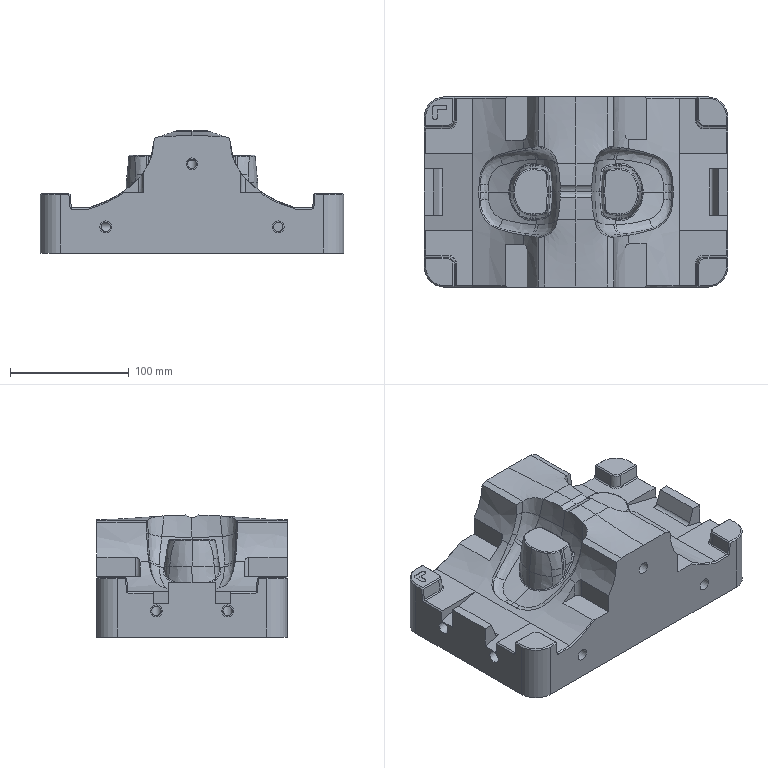NC program | NX | posted with a generic post | part box 255 x 160 x 102.619 mm
Lines 1 to 981 of 55104:
N10 G17 G21 G94 G90
(CAVITY_MILL , TOOL : D30R5)
N12 T00 M6
N14 G54
N16 G17 G0 G90 X177.095 Y-14.998 S1500 M3
N18 G43 Z115. H0
N20 Z102.321
N22 G94 G1 Z102.121 F1800.
N24 Y1.322
N26 X10.431
N28 G2 X1.322 Y10.429 R17.
N30 G1 Y149.575
N32 G2 X10.431 Y158.681 R17.
N34 G1 X244.569
N36 G2 X253.678 Y149.575 R17.
N38 G1 Y10.429
N40 G2 X244.569 Y1.322 R17.
N42 G1 X177.095
N44 Y15.322
N46 X15.322
N48 Y144.681
N50 X239.678
N52 Y15.322
N54 X177.095
N56 Y29.322
N58 X29.322
N60 Y130.681
N62 X225.678
N64 Y29.322
N66 X177.095
N68 Y43.322
N70 X43.322
N72 Y116.681
N74 X98.445
N76 Y102.681
N78 G3 X98.293 Y97.004 R56.063
N80 G1 X98.589 Y84.666
N82 G3 X99.438 Y79.957 R15.536
N84 X98.536 Y73.276 R18.646
N86 X98.46 Y57.322 R148.96
N88 G1 X57.322
N90 Y102.681
N92 X98.445
N94 X84.488 Y88.681
N96 X84.593 Y84.33
N98 G3 X85.029 Y79.931 R29.536
N100 X84.523 Y73.439 R32.646
N102 X84.422 Y71.322 R162.96
N104 G1 X71.322
N106 Y88.681
N108 X84.488
N110 X98.445 Y102.681
N112 Y116.681
N114 X211.678
N116 Y43.322
N118 X177.095
N120 Y57.322
N122 X156.555
N124 G3 X156.707 Y62.999 R56.064
N126 G1 X156.411 Y75.338
N128 G3 X155.562 Y80.046 R15.536
N130 X156.464 Y86.727 R18.646
N132 X156.538 Y102.681 R148.12
N134 G1 X153.741 Y102.543
N136 G2 X153.659 Y86.737 R145.32
N138 X152.574 Y80.012 R15.846
N140 X153.612 Y75.271 R12.736
N142 G1 X153.908 Y62.932
N144 G2 X153.69 Y56.679 R53.264
N146 X142.632 Y46.609 R11.109
N148 G1 X112.375 Y46.603
N150 G2 X101.272 Y57.153 R11.115
N152 X101.341 Y73.266 R146.16
N154 X102.426 Y79.991 R15.846
N156 X101.388 Y84.733 R12.736
N158 G1 X101.092 Y97.071
N160 G2 X101.31 Y103.324 R53.263
N162 X112.369 Y113.394 R11.108
N164 G1 X142.63 Y113.398
N166 G2 X153.726 Y102.859 R11.109
N168 X153.741 Y102.543 R145.32
N170 G1 X156.538 Y102.681
N172 X197.678
N174 Y57.322
N176 X177.095
N178 Y71.322
N180 X170.512
N182 X170.407 Y75.673
N184 G3 X169.971 Y80.072 R29.536
N186 X170.477 Y86.563 R32.646
N188 X170.578 Y88.681 R162.12
N190 G1 X183.678
N192 Y71.322
N194 X177.095
N196 Y56.322
N198 Z102.321
N200 G0 Z102.92
N202 Y-14.998
N204 Z101.821
N206 G1 Z101.621
N208 Y0.502
N210 X12.905
N212 G2 X0.502 Y12.901 R17.
N214 G1 Y147.103
N216 G2 X12.905 Y159.501 R17.
N218 G1 X242.095
N220 G2 X254.498 Y147.103 R17.
N222 G1 Y12.901
N224 G2 X242.095 Y0.502 R17.
N226 G1 X177.095
N228 Y14.502
N230 X15.341
N232 G2 X14.502 Y15.34 R3.
N234 G1 Y144.663
N236 G2 X15.341 Y145.501 R3.
N238 G1 X239.659
N240 G2 X240.498 Y144.663 R3.
N242 G1 Y15.34
N244 G2 X239.659 Y14.502 R3.
N246 G1 X177.095
N248 Y28.502
N250 X28.502
N252 Y131.501
N254 X101.002
N256 Y117.501
N258 G3 X96.735 Y106.436 R15.365
N260 G1 X96.799 Y104.162
N262 X96.803 Y104.064
N264 G2 X97.893 Y84.247 R872.408
N266 G3 X98.673 Y79.993 R15.74
N268 X97.894 Y75.752 R15.657
N270 G1 X97.557 Y68.018
N272 X97.482 Y66.698
N274 X96.8 Y55.879
N276 X96.797 Y55.778
N278 X96.772 Y52.822
N280 G3 X100.983 Y42.502 R14.442
N282 G1 X42.502
N284 Y117.501
N286 X101.002
N288 X82.814 Y103.501
N290 X82.825 Y103.27
N292 G2 X83.906 Y83.638 R858.408
N294 G3 X84.29 Y79.995 R29.74
N296 X83.907 Y76.36 R29.657
N298 G1 X83.507 Y67.537
N300 X82.831 Y56.811
N302 G3 X82.814 Y56.502 R16.8
N304 G1 X73.422
N306 Y66.502
N308 X66.502
N310 Y93.501
N312 X73.404
N314 G2 X73.915 Y83.202 R848.408
N316 G3 X74.186 Y79.995 R39.74
N318 X73.917 Y76.805 R39.657
N320 G1 X73.521 Y68.078
N322 X73.422 Y66.502
N324 Y56.502
N326 X56.502
N328 Y103.501
N330 X82.814
N332 X101.002 Y117.501
N334 Y131.501
N336 X226.498
N338 Y28.502
N340 X177.095
N342 Y42.502
N344 X153.998
N346 G3 X158.265 Y53.567 R15.365
N348 G1 X158.201 Y55.841
N350 X158.197 Y55.939
N352 G2 X157.107 Y75.756 R872.408
N354 G3 X156.327 Y80.01 R15.74
N356 X157.106 Y84.251 R15.657
N358 G1 X157.443 Y91.984
N360 X157.519 Y93.304
N362 X158.2 Y104.124
N364 X158.203 Y104.225
N366 X158.228 Y107.18
N368 G3 X154.017 Y117.501 R14.443
N370 G1 X152.033 Y115.525
N372 G2 X155.428 Y107.205 R11.643
N374 G1 X155.403 Y104.249
N376 X154.724 Y93.472
N378 X154.647 Y92.125
N380 X154.309 Y84.373
N382 G2 X153.342 Y80.011 R12.857
N384 X154.31 Y75.634 R12.94
N386 G3 X155.403 Y55.754 R875.208
N388 G1 X155.466 Y53.489
N390 G2 X150.436 Y43.076 R12.565
N392 X141.06 Y40.312 R24.234
N394 G1 X134.577 Y39.769
N396 G2 X108.878 Y41.291 R90.461
N398 X99.572 Y52.798 R11.642
N400 G1 X99.597 Y55.754
N402 X100.277 Y66.531
N404 X100.353 Y67.878
N406 X100.691 Y75.63
N408 G2 X101.658 Y79.992 R12.857
N410 X100.69 Y84.369 R12.94
N412 G3 X99.597 Y104.249 R875.208
N414 G1 X99.534 Y106.515
N416 G2 X104.564 Y116.927 R12.565
N418 X114.012 Y119.695 R24.228
N420 G1 X120.96 Y120.254
N422 G2 X146.132 Y118.71 R89.338
N424 X152.033 Y115.525 R11.643
N426 G1 X154.017 Y117.501
N428 X212.498
N430 Y42.502
N432 X177.095
N434 Y56.502
N436 X172.186
N438 X172.175 Y56.733
N440 G2 X171.094 Y76.365 R858.408
N442 G3 X170.71 Y80.008 R29.74
N444 X171.093 Y83.642 R29.657
N446 G1 X171.494 Y92.462
N448 X172.169 Y103.193
N450 G3 X172.186 Y103.501 R16.8
N452 G1 X198.498
N454 Y93.501
N456 X188.498
N458 Y66.502
N460 X181.596
N462 G2 X181.085 Y76.801 R848.408
N464 G3 X180.814 Y80.008 R39.74
N466 X181.083 Y83.197 R39.657
N468 G1 X181.48 Y91.921
N470 X181.579 Y93.501
N472 X188.498
N474 X198.498
N476 Y56.502
N478 X177.095
N480 Y41.502
N482 Z101.821
N484 G0 Z102.421
N486 Y-14.998
N488 Z101.322
N490 G1 Z101.122
N492 Y0.002
N494 X17.
N496 G2 X0. Y17.002 R17.
N498 G1 Y143.002
N500 G2 X17. Y160.002 R17.
N502 G1 X238.
N504 G2 X255. Y143.002 R17.
N506 G1 Y17.002
N508 G2 X238. Y0.002 R17.
N510 G1 X177.095
N512 Y14.002
N514 X17.
N516 G2 X14. Y17.002 R3.
N518 G1 Y143.002
N520 G2 X17. Y146.002 R3.
N522 G1 X238.
N524 G2 X241. Y143.002 R3.
N526 G1 Y17.002
N528 G2 X238. Y14.002 R3.
N530 G1 X177.095
N532 Y28.002
N534 X28.
N536 Y132.002
N538 X97.508
N540 Y118.002
N542 G3 X95.334 Y107.532 R15.873
N544 G2 X97.346 Y84.42 R222.849
N546 G3 X98.109 Y79.993 R16.551
N548 X97.346 Y75.576 R16.485
N550 G2 X95.335 Y52.474 R222.602
N552 G3 X97.508 Y42.002 R15.875
N554 G1 X42.
N556 Y118.002
N558 X97.508
N560 X81.685 Y104.002
N562 G2 X83.354 Y83.934 R208.849
N564 G3 X83.748 Y79.995 R30.551
N566 X83.355 Y76.062 R30.485
N568 G2 X82.687 Y65.13 R208.602
N570 G1 X72.725 Y66.002
N572 X66.
N574 Y94.002
N576 X72.724
N578 G2 X73.36 Y83.587 R198.849
N580 G3 X73.645 Y79.995 R40.551
N582 X73.361 Y76.41 R40.485
N584 G2 X72.725 Y66.002 R198.602
N586 G1 X82.687 Y65.13
N588 G2 X81.686 Y56.002 R208.602
N590 G1 X56.
N592 Y104.002
N594 X81.685
N596 X97.508 Y118.002
N598 Y132.002
N600 X227.
N602 Y28.002
N604 X177.095
N606 Y42.002
N608 X157.492
N610 G3 X159.666 Y52.471 R15.873
N612 G2 X157.654 Y75.583 R222.848
N614 G3 X156.891 Y80.01 R16.552
N616 X157.654 Y84.427 R16.49
N618 G2 X159.665 Y107.53 R222.815
N620 G3 X157.492 Y118.002 R15.875
N622 G1 X155.102 Y116.542
N624 G2 X156.892 Y107.918 R13.075
N626 G3 X154.856 Y84.524 R225.615
N628 G2 X153.922 Y80.011 R13.69
N630 X154.856 Y75.486 R13.752
N632 G3 X156.893 Y52.084 R225.648
N634 G2 X153.094 Y40.936 R13.073
N636 X124.802 Y33.091 R49.203
N638 X101.906 Y40.936 R50.384
N640 X98.108 Y52.086 R13.075
N642 G3 X100.145 Y75.479 R225.402
N644 G2 X101.078 Y79.992 R13.685
N646 X100.144 Y84.518 R13.751
N648 G3 X98.107 Y107.919 R225.649
N650 G2 X101.906 Y119.067 R13.073
N652 X130.198 Y126.913 R49.203
N654 X153.094 Y119.067 R50.354
N656 X155.102 Y116.542 R13.075
N658 G1 X157.492 Y118.002
N660 X213.
N662 Y42.002
N664 X177.095
N666 Y56.002
N668 X173.315
N670 G2 X171.646 Y76.069 R208.848
N672 G3 X171.252 Y80.009 R30.552
N674 X171.645 Y83.94 R30.49
N676 G2 X173.314 Y104.002 R208.815
N678 G1 X199.
N680 Y56.002
N682 X189.
N684 Y66.002
N686 X182.276
N688 G2 X181.64 Y76.416 R198.848
N690 G3 X181.355 Y80.009 R40.552
N692 X181.639 Y83.592 R40.49
N694 G2 X182.275 Y94.002 R198.815
N696 G1 X189.
N698 Y66.002
N700 Y56.002
N702 X177.095
N704 Y41.002
N706 Z101.322
N708 G0 Z101.921
N710 Y-14.998
N712 Z100.823
N714 G1 Z100.623
N716 Y0.002
N718 X17.
N720 G2 X0. Y17.002 R17.
N722 G1 Y143.002
N724 G2 X17. Y160.002 R17.
N726 G1 X238.
N728 G2 X255. Y143.002 R17.
N730 G1 Y17.002
N732 G2 X238. Y0.002 R17.
N734 G1 X177.095
N736 Y14.002
N738 X17.
N740 G2 X14. Y17.002 R3.
N742 G1 Y143.002
N744 G2 X17. Y146.002 R3.
N746 G1 X112.205
N748 Y132.002
N750 G3 X99.377 Y123.983 R57.105
N752 X94.053 Y108.951 R15.535
N754 G1 X95.365 Y102.435
N756 G2 X96.953 Y84.27 R187.108
N758 G3 X97.688 Y79.993 R16.509
N760 X96.953 Y75.712 R16.413
N762 G2 X95.521 Y58.803 R179.834
N764 G1 X95.362 Y57.559
N766 X94.275 Y52.233
N768 X94.023 Y50.9
N770 G3 X97.579 Y37.734 R15.35
N772 X97.787 Y37.522 R2.8
N774 X112.166 Y28.002 R55.65
N776 G1 X122.48 Y24.221
N778 X112.166 Y28.002
N780 X28.
N782 Y132.002
N784 X112.205
N786 X122.531 Y135.778
N788 X112.205 Y132.002
N790 X80.361 Y118.002
N792 G3 X80.329 Y106.189 R29.535
N794 G1 X81.552 Y100.112
N796 G2 X82.963 Y83.732 R173.108
N798 G3 X83.338 Y79.994 R30.509
N800 X82.963 Y76.234 R30.413
N802 G2 X81.638 Y60.61 R165.834
N804 G1 X81.541 Y59.85
N806 X80.556 Y55.022
N808 X80.528 Y54.882
N810 X80.277 Y53.555
N812 G3 X80.327 Y42.002 R29.35
N814 G1 X42.
N816 Y118.002
N818 X80.361
N820 X66.492 Y104.002
N822 G3 X66.604 Y103.427 R43.535
N824 G1 X67.735 Y97.806
N826 G2 X68.973 Y83.194 R159.108
N828 G3 X69.212 Y79.994 R44.509
N830 X68.972 Y76.756 R44.413
N832 G2 X67.755 Y62.419 R151.834
N834 G1 X67.72 Y62.141
N836 X66.828 Y57.772
N838 X66.781 Y57.532
N840 X66.529 Y56.199
N842 X66.491 Y56.002
N844 X56.
N846 Y104.002
N848 X66.492
N850 X80.361 Y118.002
N852 X112.205 Y132.002
N854 Y146.002
N856 X238.
N858 G2 X241. Y143.002 R3.
N860 G1 Y17.002
N862 G2 X238. Y14.002 R3.
N864 G1 X177.095
N866 Y28.002
N868 X142.811
N870 X132.494 Y24.223
N872 X142.811 Y28.002
N874 G3 X155.952 Y36.341 R56.515
N876 X161.141 Y49.622 R15.015
N878 G1 X161.008 Y50.707
N880 G3 X160.973 Y50.918 R2.8
N882 G1 X159.635 Y57.568
N884 G2 X158.047 Y75.733 R187.108
N886 G3 X157.312 Y80.011 R16.51
N888 X158.047 Y84.297 R16.483
N890 G2 X159.479 Y101.2 R181.155
N892 G1 X159.638 Y102.444
N894 X160.725 Y107.771
N896 X160.977 Y109.104
N898 G3 X157.421 Y122.269 R15.35
N900 X157.212 Y122.482 R2.8
N902 X142.827 Y132.002 R55.664
N904 G1 X132.509 Y135.782
N906 X142.827 Y132.002
N908 X141.662 Y129.455
N910 G2 X155.324 Y120.414 R52.864
N912 X158.228 Y109.638 R12.55
N914 G1 X157.974 Y108.29
N916 X156.874 Y102.902
N918 X156.702 Y101.555
N920 G3 X155.249 Y84.403 R183.955
N922 G2 X154.349 Y80.012 R13.683
N924 X155.249 Y75.626 R13.71
N926 G3 X156.873 Y57.101 R189.908
N928 G1 X158.229 Y50.366
N930 X158.362 Y49.281
N932 G2 X154.141 Y38.476 R12.215
N934 X127.5 Y26.335 R53.715
N936 X99.676 Y39.589 R52.85
N938 X96.772 Y50.366 R12.55
N940 G1 X97.026 Y51.713
N942 X98.126 Y57.101
N944 X98.298 Y58.448
N946 G3 X99.751 Y75.607 R182.634
N948 G2 X100.651 Y79.991 R13.613
N950 X99.751 Y84.377 R13.709
N952 G3 X98.127 Y102.902 R189.908
N954 G1 X96.798 Y109.504
N956 G2 X101.162 Y121.827 R12.735
N958 X127.5 Y133.663 R54.305
N960 X141.662 Y129.455 R52.864
N962 G1 X142.827 Y132.002
N964 X227.
N966 Y28.002
N968 X177.095
N970 Y42.002
N972 X174.67
N974 G3 X175.036 Y51.331 R29.015
N976 G1 X174.903 Y52.415
N978 G3 X174.698 Y53.68 R16.8
N980 G1 X173.448 Y59.891
N982 G2 X172.037 Y76.271 R173.108
N984 G3 X171.662 Y80.011 R30.51
N986 X172.037 Y83.77 R30.483
N988 G2 X173.362 Y99.396 R167.155
N990 G1 X173.459 Y100.153
N992 X174.444 Y104.98
N994 X174.472 Y105.121
N996 X174.723 Y106.448
N998 G3 X174.673 Y118.002 R29.35
N1000 G1 X213.
N1002 Y42.002
N1004 X177.095
N1006 X188.508 Y56.002
N1008 G3 X188.423 Y56.442 R30.8
N1010 G1 X187.265 Y62.197
N1012 G2 X186.027 Y76.809 R159.108
N1014 G3 X185.788 Y80.012 R44.51
N1016 X186.027 Y83.243 R44.483
N1018 G2 X187.245 Y97.59 R153.155
N1020 G1 X187.28 Y97.863
N1022 X188.172 Y102.23
N1024 X188.219 Y102.471
N1026 X188.471 Y103.804
N1028 X188.509 Y104.002
N1030 X199.
N1032 Y56.002
N1034 X188.508
N1036 Y41.002
N1038 Z100.823
N1040 G0 Z101.422
N1042 X177.095 Y-14.998
N1044 Z100.324
N1046 G1 Z100.124
N1048 Y0.002
N1050 X17.
N1052 G2 X0. Y17.002 R17.
N1054 G1 Y143.002
N1056 G2 X17. Y160.002 R17.
N1058 G1 X238.
N1060 G2 X255. Y143.002 R17.
N1062 G1 Y17.002
N1064 G2 X238. Y0.002 R17.
N1066 G1 X177.095
N1068 Y14.002
N1070 X17.
N1072 G2 X14. Y17.002 R3.
N1074 G1 Y143.002
N1076 G2 X17. Y146.002 R3.
N1078 G1 X103.851
N1080 Y132.002
N1082 G3 X93.864 Y120.584 R52.059
N1084 X93.638 Y120.158 R2.8
N1086 X93.408 Y107.403 R17.11
N1088 G2 X95.051 Y101.167 R30.354
N1090 X96.641 Y84.283 R148.196
N1092 G3 X97.368 Y79.978 R16.747
N1094 X96.626 Y75.493 R18.
N1096 G2 X94.859 Y57.615 R147.007
N1098 X93.447 Y52.701 R36.526
N1100 G3 X93.638 Y39.845 R17.11
N1102 X93.864 Y39.419 R2.8
N1104 X103.851 Y28.002 R52.111
N1106 G1 X28.
N1108 Y132.002
N1110 X103.851
N1112 X78.615 Y118.002
N1114 G3 X80.325 Y102.419 R31.11
N1116 G2 X81.21 Y99.059 R16.354
N1118 X82.65 Y83.77 R134.196
N1120 G3 X83.029 Y79.958 R30.747
N1122 X82.636 Y76.016 R32.
N1124 G2 X81.098 Y60.221 R133.007
N1126 X80.331 Y57.6 R22.526
N1128 G3 X78.615 Y42.002 R31.11
N1130 G1 X42.
N1132 Y118.002
N1134 X78.615
N1136 X65.297 Y104.002
N1138 G3 X67.242 Y97.435 R45.11
N1140 G2 X67.37 Y96.951 R2.354
N1142 X68.659 Y83.257 R120.196
N1144 G3 X68.902 Y79.964 R44.747
N1146 X68.646 Y76.539 R46.
N1148 G2 X67.357 Y62.97 R119.007
N1150 X67.188 Y62.424 R8.526
N1152 G3 X65.297 Y56.002 R45.11
N1154 G1 X56.
N1156 Y104.002
N1158 X65.297
N1160 X78.615 Y118.002
N1162 X103.851 Y132.002
N1164 Y146.002
N1166 X238.
N1168 G2 X241. Y143.002 R3.
N1170 G1 Y17.002
N1172 G2 X238. Y14.002 R3.
N1174 G1 X177.095
N1176 Y28.002
N1178 X151.151
N1180 G3 X161.136 Y39.419 R52.093
N1182 X161.362 Y39.845 R2.8
N1184 X161.592 Y52.6 R17.11
N1186 G2 X159.949 Y58.837 R30.36
N1188 X158.359 Y75.72 R148.196
N1190 G3 X157.636 Y80.012 R16.747
N1192 X158.36 Y84.301 R16.829
N1194 G2 X160.141 Y102.39 R150.257
N1196 X161.553 Y107.302 R36.547
N1198 G3 X161.362 Y120.158 R17.11
N1200 X161.136 Y120.584 R2.8
N1202 X151.147 Y132.002 R52.078
N1204 G1 X149.331 Y129.871
N1206 G2 X158.783 Y119.067 R49.278
N1208 X158.933 Y108.29 R14.31
N1210 G3 X157.387 Y102.902 R39.347
N1212 X155.562 Y84.406 R153.057
N1214 G2 X154.68 Y80.011 R14.029
N1216 X155.561 Y75.617 R13.947
N1218 G3 X157.181 Y58.415 R150.996
N1220 X158.975 Y51.604 R33.16
N1222 G2 X158.783 Y40.936 R14.31
N1224 X127.5 Y19.402 R49.293
N1226 X96.217 Y40.936 R49.311
N1228 X96.067 Y51.713 R14.31
N1230 G3 X97.613 Y57.101 R39.326
N1232 X99.424 Y75.389 R149.807
N1234 G2 X100.32 Y79.992 R15.2
N1236 X99.439 Y84.386 R13.947
N1238 G3 X97.819 Y101.589 R150.996
N1240 X96.025 Y108.399 R33.154
N1242 G2 X96.217 Y119.067 R14.31
N1244 X127.5 Y140.591 R49.259
N1246 X149.331 Y129.871 R49.278
N1248 G1 X151.147 Y132.002
N1250 X227.
N1252 Y28.002
N1254 X177.095
N1256 Y42.002
N1258 X176.385
N1260 G3 X174.675 Y57.584 R31.11
N1262 G2 X173.79 Y60.945 R16.36
N1264 X172.35 Y76.233 R134.196
N1266 G3 X171.977 Y80.014 R30.747
N1268 X172.35 Y83.774 R30.829
N1270 G2 X173.903 Y99.789 R136.257
N1272 X174.669 Y102.404 R22.547
N1274 G3 X176.385 Y118.002 R31.11
N1276 G1 X213.
N1278 Y42.002
N1280 X177.095
N1282 X189.703 Y56.002
N1284 G3 X187.758 Y62.568 R45.11
N1286 G2 X187.63 Y63.053 R2.36
N1288 X186.341 Y76.746 R120.196
N1290 G3 X186.101 Y80.013 R44.747
N1292 X186.34 Y83.247 R44.829
N1294 G2 X187.645 Y97.041 R122.257
N1296 X187.812 Y97.579 R8.547
N1298 G3 X189.703 Y104.002 R45.11
N1300 G1 X199.
N1302 Y56.002
N1304 X189.703
N1306 Y41.002
N1308 Z100.324
N1310 G0 Z100.923
N1312 X177.095 Y-14.998
N1314 Z99.824
N1316 G1 Z99.624
N1318 Y0.002
N1320 X17.
N1322 G2 X0. Y17.002 R17.
N1324 G1 Y143.002
N1326 G2 X17. Y160.002 R17.
N1328 G1 X113.705
N1330 Y146.002
N1332 G3 X94.061 Y124.96 R50.569
N1334 X90.853 Y113.485 R17.766
N1336 X90.881 Y113.24 R2.8
N1338 X93.279 Y105.771 R25.668
N1340 G2 X94.706 Y101.131 R16.658
N1342 X96.369 Y84.707 R133.423
N1344 G3 X97.124 Y79.992 R18.335
N1346 X96.369 Y75.327 R18.601
N1348 G2 X94.712 Y58.902 R132.904
N1350 X93.29 Y54.267 R16.422
N1352 G3 X91.547 Y49.889 R37.565
N1354 X93.046 Y36.907 R15.603
N1356 X114.003 Y14.002 R52.503
N1358 G1 X17.
N1360 G2 X14. Y17.002 R3.
N1362 G1 Y143.002
N1364 G2 X17. Y146.002 R3.
N1366 G1 X113.705
N1368 X81.925 Y132.002
N1370 G3 X76.887 Y112.515 R31.766
N1372 X77.054 Y111.047 R16.8
N1374 X80.668 Y99.689 R39.668
N1376 G2 X80.879 Y98.935 R2.658
N1378 X82.377 Y84.225 R119.423
N1380 G3 X82.789 Y79.987 R32.335
N1382 X82.378 Y75.833 R32.601
N1384 G2 X80.882 Y61.078 R118.904
N1386 X80.647 Y60.278 R2.422
N1388 G3 X78.243 Y54.249 R51.565
N1390 X80.673 Y30.33 R29.603
N1392 X81.857 Y28.002 R66.503
N1394 G1 X28.
N1396 Y132.002
N1398 X81.925
N1400 X62.928 Y118.002
N1402 G3 X62.92 Y111.544 R45.766
N1404 X63.227 Y108.854 R30.8
N1406 X67.29 Y95.241 R53.668
N1408 G2 X68.386 Y83.725 R105.423
N1410 G3 X68.659 Y79.987 R46.335
N1412 X68.388 Y76.348 R46.601
N1414 G2 X67.285 Y64.722 R104.904
N1416 G3 X64.939 Y58.608 R65.565
N1418 X63.14 Y50.7 R43.603
N1420 G1 X53.225 Y52.002
N1422 X52.
N1424 Y108.002
N1426 X53.243
N1428 G3 X53.35 Y107.287 R40.8
N1430 X57.584 Y92.481 R63.668
N1432 G2 X58.393 Y83.36 R95.423
N1434 G3 X58.606 Y79.988 R56.335
N1436 X58.395 Y76.72 R56.601
N1438 G2 X57.578 Y67.463 R94.904
N1440 G3 X55.435 Y61.72 R75.565
N1442 X53.225 Y52.002 R53.603
N1444 G1 X63.14 Y50.7
N1446 G3 X62.874 Y42.002 R43.603
N1448 G1 X42.
N1450 Y118.002
N1452 X62.928
N1454 X81.925 Y132.002
N1456 X113.705 Y146.002
N1458 Y160.002
N1460 X238.
N1462 G2 X255. Y143.002 R17.
N1464 G1 Y17.002
N1466 G2 X238. Y0.002 R17.
N1468 G1 X177.095
N1470 Y14.002
N1472 X141.289
N1474 G3 X160.94 Y35.045 R50.403
N1476 X164.147 Y46.518 R17.766
N1478 X164.119 Y46.763 R2.8
N1480 X161.721 Y54.232 R25.668
N1482 G2 X160.294 Y58.872 R16.658
N1484 X158.631 Y75.296 R133.396
N1486 G3 X157.876 Y80.011 R18.335
N1488 X158.631 Y84.676 R18.6
N1490 G2 X160.344 Y101.44 R132.904
N1492 X161.355 Y104.9 R15.162
N1494 G1 X162.909 Y108.538
N1496 G3 X161.163 Y124.545 R16.666
N1498 X141.268 Y146.002 R50.797
N1500 G1 X139.85 Y143.587
N1502 G2 X158.748 Y123.108 R47.997
N1504 X160.334 Y109.638 R13.866
N1506 G1 X158.78 Y106.
N1508 G3 X157.582 Y101.901 R17.962
N1510 X155.832 Y84.775 R135.704
N1512 G2 X154.932 Y80.009 R15.8
N1514 X155.832 Y75.203 R15.535
N1516 G3 X157.526 Y58.448 R136.196
N1518 X159.205 Y53.002 R19.458
N1520 G2 X161.354 Y46.324 R22.868
N1522 X158.531 Y36.489 R14.966
N1524 X127.5 Y11.346 R47.603
N1526 X95.513 Y38.242 R49.703
N1528 X94.208 Y49.018 R12.803
N1530 X95.817 Y53.06 R34.765
N1532 G3 X97.475 Y58.448 R19.222
N1534 X99.168 Y75.228 R135.704
N1536 G2 X100.068 Y79.995 R15.801
N1538 X99.168 Y84.8 R15.535
N1540 G3 X97.474 Y101.555 R136.223
N1542 X95.795 Y107.002 R19.458
N1544 G2 X93.646 Y113.679 R22.868
N1546 X96.469 Y123.514 R14.966
N1548 X127.5 Y148.683 R47.769
N1550 X139.85 Y143.587 R47.997
N1552 G1 X141.268 Y146.002
N1554 X238.
N1556 G2 X241. Y143.002 R3.
N1558 G1 Y17.002
N1560 G2 X238. Y14.002 R3.
N1562 G1 X177.095
N1564 Y28.002
N1566 X173.075
N1568 G3 X178.113 Y47.489 R31.766
N1570 X177.946 Y48.956 R16.8
N1572 X174.332 Y60.314 R39.668
N1574 G2 X174.121 Y61.068 R2.658
N1576 X172.623 Y75.778 R119.396
N1578 G3 X172.211 Y80.016 R32.335
N1580 X172.622 Y84.17 R32.6
N1582 G2 X174.153 Y99.137 R118.904
N1584 X174.23 Y99.402 R1.162
N1586 G1 X175.828 Y103.144
N1588 G3 X173.288 Y131.6 R30.666
N1590 G1 X173.081 Y132.002
N1592 X227.
N1594 Y28.002
N1596 X177.095
N1598 X192.072 Y42.002
N1600 G3 X192.08 Y48.459 R45.766
N1602 X191.773 Y51.149 R30.8
N1604 X187.71 Y64.763 R53.668
N1606 G2 X186.614 Y76.278 R105.396
N1608 G3 X186.341 Y80.016 R46.335
N1610 X186.612 Y83.655 R46.6
N1612 G2 X187.727 Y95.359 R104.904
N1614 G1 X188.726 Y97.698
N1616 G3 X192.092 Y118.002 R44.666
N1618 G1 X213.
N1620 Y52.002
N1622 X203.
N1624 X201.757
N1626 G3 X201.65 Y52.716 R40.8
N1628 X197.416 Y67.522 R63.668
N1630 G2 X196.607 Y76.643 R95.396
N1632 G3 X196.394 Y80.015 R56.335
N1634 X196.605 Y83.284 R56.6
N1636 G2 X197.435 Y92.63 R94.904
N1638 G1 X197.923 Y93.772
N1640 G3 X201.751 Y108.002 R54.666
N1642 G1 X203.
N1644 Y52.002
N1646 X213.
N1648 Y42.002
N1650 X192.072
N1652 Y27.002
N1654 Z99.824
N1656 G0 Z100.424
N1658 X177.095 Y-14.998
N1660 Z99.325
N1662 G1 Z99.125
N1664 Y0.002
N1666 X17.
N1668 G2 X0. Y17.002 R17.
N1670 G1 Y143.002
N1672 G2 X17. Y160.002 R17.
N1674 G1 X102.311
N1676 Y146.002
N1678 G3 X91.117 Y124.095 R57.328
N1680 X89.321 Y114.975 R22.029
N1682 X89.347 Y114.644 R2.8
N1684 X92.757 Y105.521 R22.217
N1686 G2 X94.438 Y101.077 R12.576
N1688 X96.214 Y84.27 R130.715
N1690 G3 X96.919 Y79.988 R17.733
N1692 X96.233 Y76.172 R19.028
N1694 G1 X96.227 Y76.067
N1696 G2 X94.423 Y58.825 R131.139
N1698 X93.194 Y55.298 R11.376
N1700 G1 X91.318 Y51.866
N1702 G3 X90.183 Y38.776 R16.142
N1704 X102.51 Y14.002 R66.75
N1706 G1 X17.
N1708 G2 X14. Y17.002 R3.
N1710 G1 Y143.002
N1712 G2 X17. Y146.002 R3.
N1714 G1 X102.311
N1716 X78.865 Y132.002
N1718 G3 X77.83 Y128.593 R71.328
N1720 X75.324 Y114.72 R36.029
N1722 X75.478 Y112.737 R16.8
N1724 X80.692 Y98.401 R36.217
N1726 G2 X82.225 Y83.702 R116.715
N1728 G3 X82.598 Y79.976 R31.733
N1730 X82.264 Y77.099 R33.028
N1732 G1 X82.243 Y76.732
N1734 G2 X80.699 Y61.628 R117.139
N1736 G1 X79.049 Y58.609
N1738 G3 X76.755 Y34.791 R30.142
N1740 X78.878 Y28.002 R80.75
N1742 G1 X28.
N1744 Y132.002
N1746 X78.865
N1748 X61.387 Y118.002
N1750 G3 X61.326 Y114.465 R50.029
N1752 X61.608 Y110.829 R30.8
N1754 X67.27 Y93.628 R50.217
N1756 G2 X68.237 Y83.135 R102.715
N1758 G3 X68.473 Y79.988 R45.733
N1760 X68.292 Y77.999 R47.028
N1762 G1 X68.257 Y77.389
N1764 X58.264 Y77.746
N1766 G2 X57.586 Y69.373 R93.139
N1768 G3 X52. Y52.737 R54.142
N1770 G1 Y107.529
N1772 G3 X57.596 Y90.546 R60.217
N1774 G2 X58.245 Y82.729 R92.715
N1776 G3 X58.423 Y80.002 R55.733
N1778 X58.316 Y78.694 R57.028
N1780 G1 X58.308 Y78.567
N1782 X58.274 Y77.957
N1784 G3 X58.264 Y77.746 R10.
N1786 G1 X68.257 Y77.389
N1788 G2 X67.247 Y66.208 R103.139
N1790 G1 X66.776 Y65.346
N1792 G3 X61.346 Y42.002 R44.142
N1794 G1 X42.
N1796 Y118.002
N1798 X61.387
N1800 X78.865 Y132.002
N1802 X102.311 Y146.002
N1804 Y160.002
N1806 X238.
N1808 G2 X255. Y143.002 R17.
N1810 G1 Y17.002
N1812 G2 X238. Y0.002 R17.
N1814 G1 X177.095
N1816 Y14.002
N1818 X152.689
N1820 G3 X163.883 Y35.908 R57.328
N1822 X165.679 Y45.028 R22.029
N1824 X165.653 Y45.359 R2.8
N1826 X162.243 Y54.482 R22.217
N1828 G2 X160.562 Y58.924 R12.591
N1830 X158.786 Y75.733 R130.679
N1832 G3 X158.083 Y80.008 R17.73
N1834 X158.788 Y84.319 R18.131
N1836 G2 X160.575 Y101.169 R131.61
N1838 X161.809 Y104.71 R11.409
N1840 G1 X163.682 Y108.137
N1842 G3 X164.817 Y121.227 R16.142
N1844 X152.49 Y146.002 R66.75
N1846 G1 X150.296 Y144.262
N1848 G2 X162.135 Y120.414 R63.95
N1850 X161.229 Y109.487 R13.342
N1852 G1 X159.352 Y106.053
N1854 G3 X157.816 Y101.643 R14.209
N1856 X155.99 Y84.434 R134.41
N1858 G2 X155.143 Y80.003 R15.331
N1860 X155.989 Y75.62 R14.93
N1862 G3 X157.803 Y58.448 R133.479
N1864 X159.88 Y52.98 R15.391
N1866 G2 X162.879 Y44.977 R19.417
N1868 X161.229 Y36.826 R19.229
N1870 X139.642 Y5.725 R54.528
N1872 X112.981 Y7.105 R21.736
N1874 X92.865 Y39.589 R63.95
N1876 X93.771 Y50.516 R13.342
N1878 G1 X95.651 Y53.955
N1880 G3 X97.183 Y58.351 R14.176
N1882 X99.025 Y75.96 R133.939
N1884 G2 X99.857 Y80. R16.228
N1886 X99.011 Y84.384 R14.933
N1888 G3 X97.197 Y101.555 R133.515
N1890 X95.12 Y107.023 R15.376
N1892 G2 X92.121 Y115.026 R19.417
N1894 X93.771 Y123.177 R19.229
N1896 X116.531 Y155.075 R54.528
N1898 X136.945 Y155.714 R19.466
N1900 G1 X142.341 Y152.618
N1902 G2 X150.296 Y144.262 R63.95
N1904 G1 X152.49 Y146.002
N1906 X238.
N1908 G2 X241. Y143.002 R3.
N1910 G1 Y17.002
N1912 G2 X238. Y14.002 R3.
N1914 G1 X177.095
N1916 Y28.002
N1918 X176.135
N1920 G3 X177.171 Y31.41 R71.328
N1922 X179.676 Y45.283 R36.029
N1924 X179.522 Y47.267 R16.8
N1926 X174.308 Y61.602 R36.217
N1928 G2 X172.775 Y76.3 R116.679
N1930 G3 X172.404 Y80.018 R31.73
N1932 X172.776 Y83.741 R32.131
N1934 G2 X174.301 Y98.375 R117.61
N1936 G1 X175.951 Y101.394
N1938 G3 X178.245 Y125.212 R30.142
N1940 X176.122 Y132.002 R80.75
N1942 G1 X227.
N1944 Y28.002
N1946 X177.095
N1948 X193.613 Y42.002
N1950 G3 X193.674 Y45.538 R50.029
N1952 X193.392 Y49.174 R30.8
N1954 X187.73 Y66.375 R50.217
N1956 G2 X186.763 Y76.868 R102.679
N1958 G3 X186.526 Y80.019 R45.73
N1960 X186.764 Y83.164 R46.131